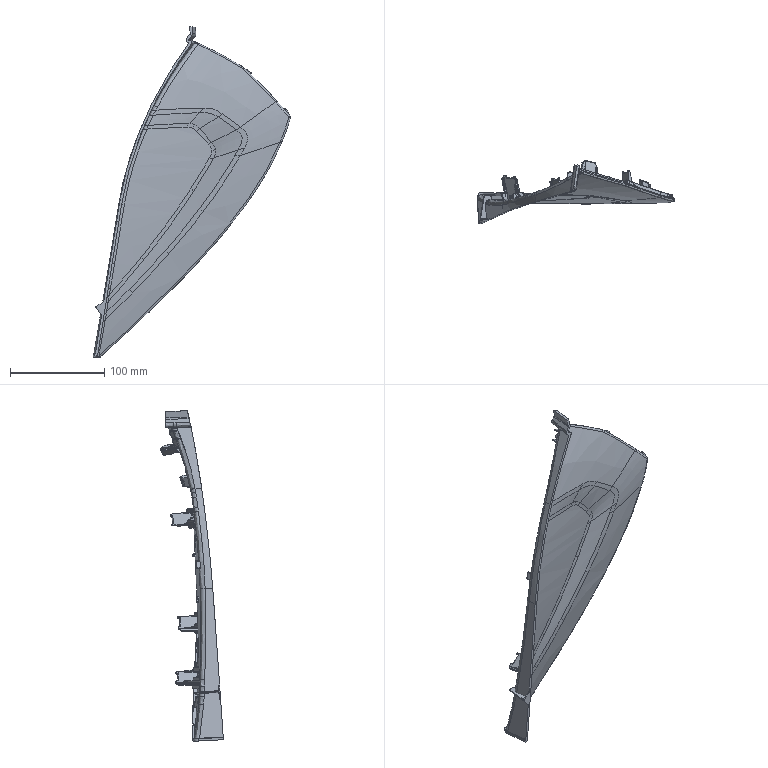Part | SolidWorks | features BaseBody 1 | 1 solid | 1833 faces | box 209.02 x 66.466 x 351.204 mm | volume 105260 mm3 | spline 1416 | cylinder 243 | plane 174 | commonest cylinder face diameters 0.6 x92 2 x49 0.5 x44 0.4 x33 1 x15 6 x4